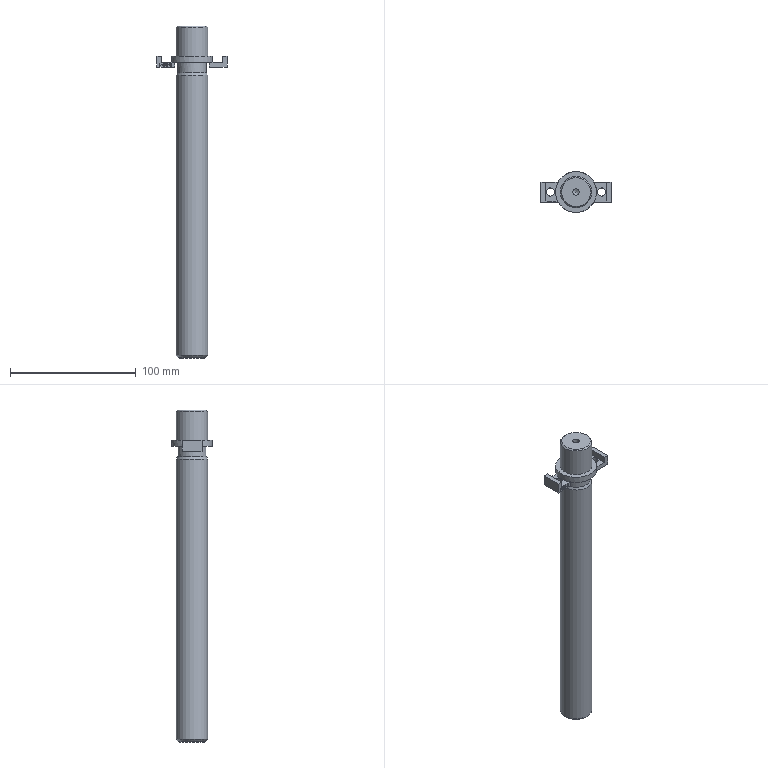Part | STEP file | lll_id4586_x_t | 1 solid | 114 faces | box 55.942 x 32.6 x 264 mm | volume 132010 mm3 | plane 66 | other 36 | cylinder 7 | cone 4 | torus 1 | commonest cylinder face diameters 6.5 x2 25 x2 5 x1 23 x1 32.6 x1